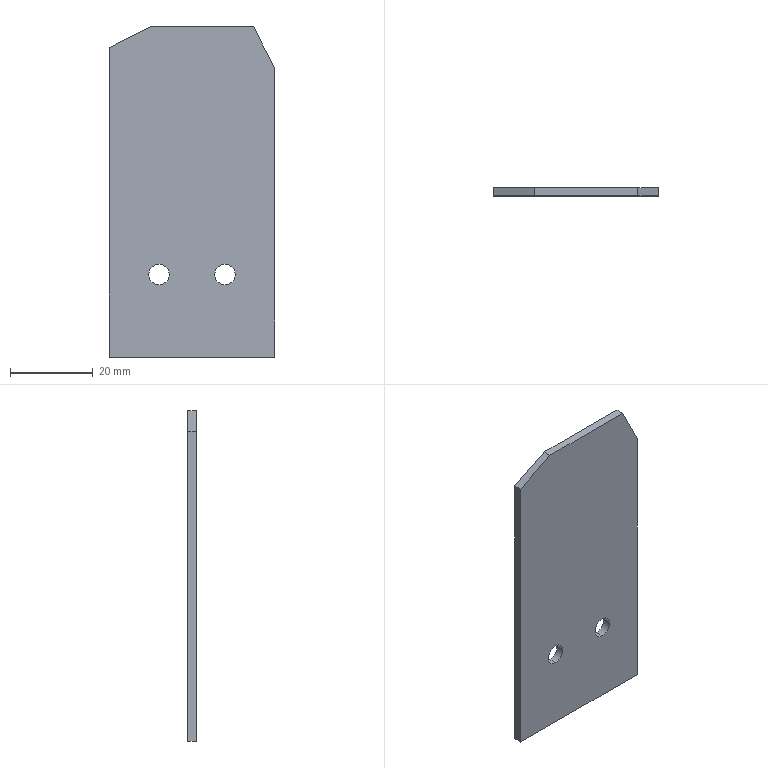Part | SolidWorks | features Chamfer 1, Cut 1, Extrusion 1 | 1 solid | 12 faces | box 40 x 2 x 80 mm | volume 6221 mm3 | plane 8 | cylinder 4 | commonest cylinder face diameters 5 x4
STEP:
#1=CARTESIAN_POINT('',(8.,2.,-22.5));
#2=VERTEX_POINT('',#1);
#3=CARTESIAN_POINT('',(8.,2.,-17.5));
#4=VERTEX_POINT('',#3);
#5=CARTESIAN_POINT('',(8.,2.,-20.));
#6=DIRECTION('',(0.,1.,0.));
#7=DIRECTION('',(0.,0.,1.));
#8=AXIS2_PLACEMENT_3D('',#5,#6,#7);
#9=CIRCLE('',#8,2.5);
#10=EDGE_CURVE('',#2,#4,#9,.T.);
#11=ORIENTED_EDGE('',*,*,#10,.T.);
#12=CARTESIAN_POINT('',(8.,0.,-17.5));
#13=VERTEX_POINT('',#12);
#14=CARTESIAN_POINT('',(8.,10.,-17.5));
#15=DIRECTION('',(0.,-1.,0.));
#16=VECTOR('',#15,1000.);
#17=LINE('',#14,#16);
#18=EDGE_CURVE('',#4,#13,#17,.T.);
#19=ORIENTED_EDGE('',*,*,#18,.T.);
#20=CARTESIAN_POINT('',(8.,0.,-22.5));
#21=VERTEX_POINT('',#20);
#22=CARTESIAN_POINT('',(8.,0.,-20.));
#23=DIRECTION('',(0.,-1.,0.));
#24=DIRECTION('',(0.,0.,-1.));
#25=AXIS2_PLACEMENT_3D('',#22,#23,#24);
#26=CIRCLE('',#25,2.5);
#27=EDGE_CURVE('',#13,#21,#26,.T.);
#28=ORIENTED_EDGE('',*,*,#27,.T.);
#29=CARTESIAN_POINT('',(8.,10.,-22.5));
#30=DIRECTION('',(0.,-1.,0.));
#31=VECTOR('',#30,1000.);
#32=LINE('',#29,#31);
#33=EDGE_CURVE('',#2,#21,#32,.T.);
#34=ORIENTED_EDGE('',*,*,#33,.F.);
#35=EDGE_LOOP('',(#11,#19,#28,#34));
#36=FACE_OUTER_BOUND('',#35,.T.);
#37=CARTESIAN_POINT('',(8.,10.,-20.));
#38=DIRECTION('',(0.,-1.,0.));
#39=DIRECTION('',(0.,0.,-1.));
#40=AXIS2_PLACEMENT_3D('',#37,#38,#39);
#41=CYLINDRICAL_SURFACE('',#40,2.5);
#42=ADVANCED_FACE('',(#36),#41,.F.);
#43=CARTESIAN_POINT('',(-8.,2.,-22.5));
#44=VERTEX_POINT('',#43);
#45=CARTESIAN_POINT('',(-8.,2.,-17.5));
#46=VERTEX_POINT('',#45);
#47=CARTESIAN_POINT('',(-8.,2.,-20.));
#48=DIRECTION('',(0.,1.,0.));
#49=DIRECTION('',(0.,0.,1.));
#50=AXIS2_PLACEMENT_3D('',#47,#48,#49);
#51=CIRCLE('',#50,2.5);
#52=EDGE_CURVE('',#44,#46,#51,.T.);
#53=ORIENTED_EDGE('',*,*,#52,.T.);
#54=CARTESIAN_POINT('',(-8.,0.,-17.5));
#55=VERTEX_POINT('',#54);
#56=CARTESIAN_POINT('',(-8.,10.,-17.5));
#57=DIRECTION('',(0.,-1.,0.));
#58=VECTOR('',#57,1000.);
#59=LINE('',#56,#58);
#60=EDGE_CURVE('',#46,#55,#59,.T.);
#61=ORIENTED_EDGE('',*,*,#60,.T.);
#62=CARTESIAN_POINT('',(-8.,0.,-22.5));
#63=VERTEX_POINT('',#62);
#64=CARTESIAN_POINT('',(-8.,0.,-20.));
#65=DIRECTION('',(0.,-1.,0.));
#66=DIRECTION('',(0.,0.,-1.));
#67=AXIS2_PLACEMENT_3D('',#64,#65,#66);
#68=CIRCLE('',#67,2.5);
#69=EDGE_CURVE('',#55,#63,#68,.T.);
#70=ORIENTED_EDGE('',*,*,#69,.T.);
#71=CARTESIAN_POINT('',(-8.,10.,-22.5));
#72=DIRECTION('',(0.,-1.,0.));
#73=VECTOR('',#72,1000.);
#74=LINE('',#71,#73);
#75=EDGE_CURVE('',#44,#63,#74,.T.);
#76=ORIENTED_EDGE('',*,*,#75,.F.);
#77=EDGE_LOOP('',(#53,#61,#70,#76));
#78=FACE_OUTER_BOUND('',#77,.T.);
#79=CARTESIAN_POINT('',(-8.,10.,-20.));
#80=DIRECTION('',(0.,-1.,0.));
#81=DIRECTION('',(0.,0.,-1.));
#82=AXIS2_PLACEMENT_3D('',#79,#80,#81);
#83=CYLINDRICAL_SURFACE('',#82,2.5);
#84=ADVANCED_FACE('',(#78),#83,.F.);
#85=CARTESIAN_POINT('',(20.,2.,30.));
#86=VERTEX_POINT('',#85);
#87=CARTESIAN_POINT('',(20.,2.,-40.));
#88=VERTEX_POINT('',#87);
#89=CARTESIAN_POINT('',(20.,2.,-40.));
#90=DIRECTION('',(0.,0.,-1.));
#91=VECTOR('',#90,1000.);
#92=LINE('',#89,#91);
#93=EDGE_CURVE('',#86,#88,#92,.T.);
#94=ORIENTED_EDGE('',*,*,#93,.F.);
#95=CARTESIAN_POINT('',(20.,0.,30.));
#96=VERTEX_POINT('',#95);
#97=CARTESIAN_POINT('',(20.,2.,30.));
#98=DIRECTION('',(0.,-1.,0.));
#99=VECTOR('',#98,1000.);
#100=LINE('',#97,#99);
#101=EDGE_CURVE('',#86,#96,#100,.T.);
#102=ORIENTED_EDGE('',*,*,#101,.T.);
#103=CARTESIAN_POINT('',(20.,0.,-40.));
#104=VERTEX_POINT('',#103);
#105=CARTESIAN_POINT('',(20.,0.,-40.));
#106=DIRECTION('',(0.,0.,-1.));
#107=VECTOR('',#106,1000.);
#108=LINE('',#105,#107);
#109=EDGE_CURVE('',#96,#104,#108,.T.);
#110=ORIENTED_EDGE('',*,*,#109,.T.);
#111=CARTESIAN_POINT('',(20.,2.,-40.));
#112=DIRECTION('',(0.,-1.,0.));
#113=VECTOR('',#112,1000.);
#114=LINE('',#111,#113);
#115=EDGE_CURVE('',#88,#104,#114,.T.);
#116=ORIENTED_EDGE('',*,*,#115,.F.);
#117=EDGE_LOOP('',(#94,#102,#110,#116));
#118=FACE_OUTER_BOUND('',#117,.T.);
#119=CARTESIAN_POINT('',(20.,2.,-40.));
#120=DIRECTION('',(-1.,0.,0.));
#121=DIRECTION('',(0.,0.,1.));
#122=AXIS2_PLACEMENT_3D('',#119,#120,#121);
#123=PLANE('',#122);
#124=ADVANCED_FACE('',(#118),#123,.F.);
#125=CARTESIAN_POINT('',(-20.,0.,-40.));
#126=VERTEX_POINT('',#125);
#127=CARTESIAN_POINT('',(-20.,0.,-40.));
#128=DIRECTION('',(-1.,0.,0.));
#129=VECTOR('',#128,1000.);
#130=LINE('',#127,#129);
#131=EDGE_CURVE('',#104,#126,#130,.T.);
#132=ORIENTED_EDGE('',*,*,#131,.T.);
#133=CARTESIAN_POINT('',(-20.,2.,-40.));
#134=VERTEX_POINT('',#133);
#135=CARTESIAN_POINT('',(-20.,2.,-40.));
#136=DIRECTION('',(0.,-1.,0.));
#137=VECTOR('',#136,1000.);
#138=LINE('',#135,#137);
#139=EDGE_CURVE('',#134,#126,#138,.T.);
#140=ORIENTED_EDGE('',*,*,#139,.F.);
#141=CARTESIAN_POINT('',(-20.,2.,-40.));
#142=DIRECTION('',(-1.,0.,0.));
#143=VECTOR('',#142,1000.);
#144=LINE('',#141,#143);
#145=EDGE_CURVE('',#88,#134,#144,.T.);
#146=ORIENTED_EDGE('',*,*,#145,.F.);
#147=ORIENTED_EDGE('',*,*,#115,.T.);
#148=EDGE_LOOP('',(#132,#140,#146,#147));
#149=FACE_OUTER_BOUND('',#148,.T.);
#150=CARTESIAN_POINT('',(-20.,2.,-40.));
#151=DIRECTION('',(0.,0.,1.));
#152=DIRECTION('',(1.,0.,0.));
#153=AXIS2_PLACEMENT_3D('',#150,#151,#152);
#154=PLANE('',#153);
#155=ADVANCED_FACE('',(#149),#154,.F.);
#156=CARTESIAN_POINT('',(-20.,0.,35.));
#157=VERTEX_POINT('',#156);
#158=CARTESIAN_POINT('',(-20.,0.,-40.));
#159=DIRECTION('',(0.,0.,1.));
#160=VECTOR('',#159,1000.);
#161=LINE('',#158,#160);
#162=EDGE_CURVE('',#126,#157,#161,.T.);
#163=ORIENTED_EDGE('',*,*,#162,.T.);
#164=CARTESIAN_POINT('',(-20.,2.,35.));
#165=VERTEX_POINT('',#164);
#166=CARTESIAN_POINT('',(-20.,2.,35.));
#167=DIRECTION('',(0.,1.,0.));
#168=VECTOR('',#167,1000.);
#169=LINE('',#166,#168);
#170=EDGE_CURVE('',#157,#165,#169,.T.);
#171=ORIENTED_EDGE('',*,*,#170,.T.);
#172=CARTESIAN_POINT('',(-20.,2.,-40.));
#173=DIRECTION('',(0.,0.,1.));
#174=VECTOR('',#173,1000.);
#175=LINE('',#172,#174);
#176=EDGE_CURVE('',#134,#165,#175,.T.);
#177=ORIENTED_EDGE('',*,*,#176,.F.);
#178=ORIENTED_EDGE('',*,*,#139,.T.);
#179=EDGE_LOOP('',(#163,#171,#177,#178));
#180=FACE_OUTER_BOUND('',#179,.T.);
#181=CARTESIAN_POINT('',(-20.,2.,-40.));
#182=DIRECTION('',(1.,0.,0.));
#183=DIRECTION('',(0.,0.,-1.));
#184=AXIS2_PLACEMENT_3D('',#181,#182,#183);
#185=PLANE('',#184);
#186=ADVANCED_FACE('',(#180),#185,.F.);
#187=CARTESIAN_POINT('',(-10.,0.,40.));
#188=VERTEX_POINT('',#187);
#189=CARTESIAN_POINT('',(15.,0.,40.));
#190=VERTEX_POINT('',#189);
#191=CARTESIAN_POINT('',(-20.,0.,40.));
#192=DIRECTION('',(1.,0.,0.));
#193=VECTOR('',#192,1000.);
#194=LINE('',#191,#193);
#195=EDGE_CURVE('',#188,#190,#194,.T.);
#196=ORIENTED_EDGE('',*,*,#195,.T.);
#197=CARTESIAN_POINT('',(15.,2.,40.));
#198=VERTEX_POINT('',#197);
#199=CARTESIAN_POINT('',(15.,2.,40.));
#200=DIRECTION('',(0.,1.,0.));
#201=VECTOR('',#200,1000.);
#202=LINE('',#199,#201);
#203=EDGE_CURVE('',#190,#198,#202,.T.);
#204=ORIENTED_EDGE('',*,*,#203,.T.);
#205=CARTESIAN_POINT('',(-10.,2.,40.));
#206=VERTEX_POINT('',#205);
#207=CARTESIAN_POINT('',(-20.,2.,40.));
#208=DIRECTION('',(1.,0.,0.));
#209=VECTOR('',#208,1000.);
#210=LINE('',#207,#209);
#211=EDGE_CURVE('',#206,#198,#210,.T.);
#212=ORIENTED_EDGE('',*,*,#211,.F.);
#213=CARTESIAN_POINT('',(-10.,2.,40.));
#214=DIRECTION('',(0.,-1.,0.));
#215=VECTOR('',#214,1000.);
#216=LINE('',#213,#215);
#217=EDGE_CURVE('',#206,#188,#216,.T.);
#218=ORIENTED_EDGE('',*,*,#217,.T.);
#219=EDGE_LOOP('',(#196,#204,#212,#218));
#220=FACE_OUTER_BOUND('',#219,.T.);
#221=CARTESIAN_POINT('',(-20.,2.,40.));
#222=DIRECTION('',(0.,0.,-1.));
#223=DIRECTION('',(-1.,0.,0.));
#224=AXIS2_PLACEMENT_3D('',#221,#222,#223);
#225=PLANE('',#224);
#226=ADVANCED_FACE('',(#220),#225,.F.);
#227=ORIENTED_EDGE('',*,*,#10,.F.);
#228=CARTESIAN_POINT('',(8.,2.,-20.));
#229=DIRECTION('',(0.,1.,0.));
#230=DIRECTION('',(0.,0.,1.));
#231=AXIS2_PLACEMENT_3D('',#228,#229,#230);
#232=CIRCLE('',#231,2.5);
#233=EDGE_CURVE('',#4,#2,#232,.T.);
#234=ORIENTED_EDGE('',*,*,#233,.F.);
#235=EDGE_LOOP('',(#227,#234));
#236=FACE_BOUND('',#235,.T.);
#237=ORIENTED_EDGE('',*,*,#52,.F.);
#238=CARTESIAN_POINT('',(-8.,2.,-20.));
#239=DIRECTION('',(0.,1.,0.));
#240=DIRECTION('',(0.,0.,1.));
#241=AXIS2_PLACEMENT_3D('',#238,#239,#240);
#242=CIRCLE('',#241,2.5);
#243=EDGE_CURVE('',#46,#44,#242,.T.);
#244=ORIENTED_EDGE('',*,*,#243,.F.);
#245=EDGE_LOOP('',(#237,#244));
#246=FACE_BOUND('',#245,.T.);
#247=ORIENTED_EDGE('',*,*,#211,.T.);
#248=CARTESIAN_POINT('',(28.,2.,14.));
#249=DIRECTION('',(0.4472,0.,-0.8944));
#250=VECTOR('',#249,1000.);
#251=LINE('',#248,#250);
#252=EDGE_CURVE('',#198,#86,#251,.T.);
#253=ORIENTED_EDGE('',*,*,#252,.T.);
#254=ORIENTED_EDGE('',*,*,#93,.T.);
#255=ORIENTED_EDGE('',*,*,#145,.T.);
#256=ORIENTED_EDGE('',*,*,#176,.T.);
#257=CARTESIAN_POINT('',(-18.,2.,36.));
#258=DIRECTION('',(0.8944,0.,0.4472));
#259=VECTOR('',#258,1000.);
#260=LINE('',#257,#259);
#261=EDGE_CURVE('',#165,#206,#260,.T.);
#262=ORIENTED_EDGE('',*,*,#261,.T.);
#263=EDGE_LOOP('',(#247,#253,#254,#255,#256,#262));
#264=FACE_OUTER_BOUND('',#263,.T.);
#265=CARTESIAN_POINT('',(0.,2.,0.));
#266=DIRECTION('',(0.,1.,0.));
#267=DIRECTION('',(0.,0.,1.));
#268=AXIS2_PLACEMENT_3D('',#265,#266,#267);
#269=PLANE('',#268);
#270=ADVANCED_FACE('',(#236,#246,#264),#269,.T.);
#271=CARTESIAN_POINT('',(8.,0.,-20.));
#272=DIRECTION('',(0.,-1.,0.));
#273=DIRECTION('',(0.,0.,-1.));
#274=AXIS2_PLACEMENT_3D('',#271,#272,#273);
#275=CIRCLE('',#274,2.5);
#276=EDGE_CURVE('',#21,#13,#275,.T.);
#277=ORIENTED_EDGE('',*,*,#276,.F.);
#278=ORIENTED_EDGE('',*,*,#27,.F.);
#279=EDGE_LOOP('',(#277,#278));
#280=FACE_BOUND('',#279,.T.);
#281=CARTESIAN_POINT('',(-8.,0.,-20.));
#282=DIRECTION('',(0.,-1.,0.));
#283=DIRECTION('',(0.,0.,-1.));
#284=AXIS2_PLACEMENT_3D('',#281,#282,#283);
#285=CIRCLE('',#284,2.5);
#286=EDGE_CURVE('',#63,#55,#285,.T.);
#287=ORIENTED_EDGE('',*,*,#286,.F.);
#288=ORIENTED_EDGE('',*,*,#69,.F.);
#289=EDGE_LOOP('',(#287,#288));
#290=FACE_BOUND('',#289,.T.);
#291=ORIENTED_EDGE('',*,*,#109,.F.);
#292=CARTESIAN_POINT('',(20.,0.,30.));
#293=DIRECTION('',(-0.4472,0.,0.8944));
#294=VECTOR('',#293,1000.);
#295=LINE('',#292,#294);
#296=EDGE_CURVE('',#96,#190,#295,.T.);
#297=ORIENTED_EDGE('',*,*,#296,.T.);
#298=ORIENTED_EDGE('',*,*,#195,.F.);
#299=CARTESIAN_POINT('',(-10.,0.,40.));
#300=DIRECTION('',(-0.8944,0.,-0.4472));
#301=VECTOR('',#300,1000.);
#302=LINE('',#299,#301);
#303=EDGE_CURVE('',#188,#157,#302,.T.);
#304=ORIENTED_EDGE('',*,*,#303,.T.);
#305=ORIENTED_EDGE('',*,*,#162,.F.);
#306=ORIENTED_EDGE('',*,*,#131,.F.);
#307=EDGE_LOOP('',(#291,#297,#298,#304,#305,#306));
#308=FACE_OUTER_BOUND('',#307,.T.);
#309=CARTESIAN_POINT('',(0.,0.,0.));
#310=DIRECTION('',(0.,1.,0.));
#311=DIRECTION('',(0.,0.,1.));
#312=AXIS2_PLACEMENT_3D('',#309,#310,#311);
#313=PLANE('',#312);
#314=ADVANCED_FACE('',(#280,#290,#308),#313,.F.);
#315=ORIENTED_EDGE('',*,*,#60,.F.);
#316=ORIENTED_EDGE('',*,*,#243,.T.);
#317=ORIENTED_EDGE('',*,*,#75,.T.);
#318=ORIENTED_EDGE('',*,*,#286,.T.);
#319=EDGE_LOOP('',(#315,#316,#317,#318));
#320=FACE_OUTER_BOUND('',#319,.T.);
#321=CARTESIAN_POINT('',(-8.,10.,-20.));
#322=DIRECTION('',(0.,-1.,0.));
#323=DIRECTION('',(0.,0.,-1.));
#324=AXIS2_PLACEMENT_3D('',#321,#322,#323);
#325=CYLINDRICAL_SURFACE('',#324,2.5);
#326=ADVANCED_FACE('',(#320),#325,.F.);
#327=ORIENTED_EDGE('',*,*,#18,.F.);
#328=ORIENTED_EDGE('',*,*,#233,.T.);
#329=ORIENTED_EDGE('',*,*,#33,.T.);
#330=ORIENTED_EDGE('',*,*,#276,.T.);
#331=EDGE_LOOP('',(#327,#328,#329,#330));
#332=FACE_OUTER_BOUND('',#331,.T.);
#333=CARTESIAN_POINT('',(8.,10.,-20.));
#334=DIRECTION('',(0.,-1.,0.));
#335=DIRECTION('',(0.,0.,-1.));
#336=AXIS2_PLACEMENT_3D('',#333,#334,#335);
#337=CYLINDRICAL_SURFACE('',#336,2.5);
#338=ADVANCED_FACE('',(#332),#337,.F.);
#339=ORIENTED_EDGE('',*,*,#252,.F.);
#340=ORIENTED_EDGE('',*,*,#203,.F.);
#341=ORIENTED_EDGE('',*,*,#296,.F.);
#342=ORIENTED_EDGE('',*,*,#101,.F.);
#343=EDGE_LOOP('',(#339,#340,#341,#342));
#344=FACE_OUTER_BOUND('',#343,.T.);
#345=CARTESIAN_POINT('',(20.,2.,30.));
#346=DIRECTION('',(-0.8944,0.,-0.4472));
#347=DIRECTION('',(0.,-1.,0.));
#348=AXIS2_PLACEMENT_3D('',#345,#346,#347);
#349=PLANE('',#348);
#350=ADVANCED_FACE('',(#344),#349,.F.);
#351=ORIENTED_EDGE('',*,*,#261,.F.);
#352=ORIENTED_EDGE('',*,*,#170,.F.);
#353=ORIENTED_EDGE('',*,*,#303,.F.);
#354=ORIENTED_EDGE('',*,*,#217,.F.);
#355=EDGE_LOOP('',(#351,#352,#353,#354));
#356=FACE_OUTER_BOUND('',#355,.T.);
#357=CARTESIAN_POINT('',(-10.,2.,40.));
#358=DIRECTION('',(0.4472,0.,-0.8944));
#359=DIRECTION('',(0.,-1.,0.));
#360=AXIS2_PLACEMENT_3D('',#357,#358,#359);
#361=PLANE('',#360);
#362=ADVANCED_FACE('',(#356),#361,.F.);
#363=CLOSED_SHELL('',(#42,#84,#124,#155,#186,#226,#270,#314,#326,#338,#350,#362));
#364=MANIFOLD_SOLID_BREP('',#363);
#365=CARTESIAN_POINT('',(0.,0.,0.));
#366=DIRECTION('',(0.,0.,1.));
#367=DIRECTION('',(1.,0.,0.));
#368=AXIS2_PLACEMENT_3D('',#365,#366,#367);
#369=(LENGTH_UNIT()NAMED_UNIT(*)SI_UNIT(.MILLI.,.METRE.));
#370=UNCERTAINTY_MEASURE_WITH_UNIT(LENGTH_MEASURE(0.00001),#369,'','');
#371=(NAMED_UNIT(*)PLANE_ANGLE_UNIT()SI_UNIT($,.RADIAN.));
#372=(NAMED_UNIT(*)SI_UNIT($,.STERADIAN.)SOLID_ANGLE_UNIT());
#373=(GEOMETRIC_REPRESENTATION_CONTEXT(3)GLOBAL_UNCERTAINTY_ASSIGNED_CONTEXT((#370))GLOBAL_UNIT_ASSIGNED_CONTEXT((#369,#371,#372))REPRESENTATION_CONTEXT('',''));
#374=ADVANCED_BREP_SHAPE_REPRESENTATION('',(#364,#368),#373);